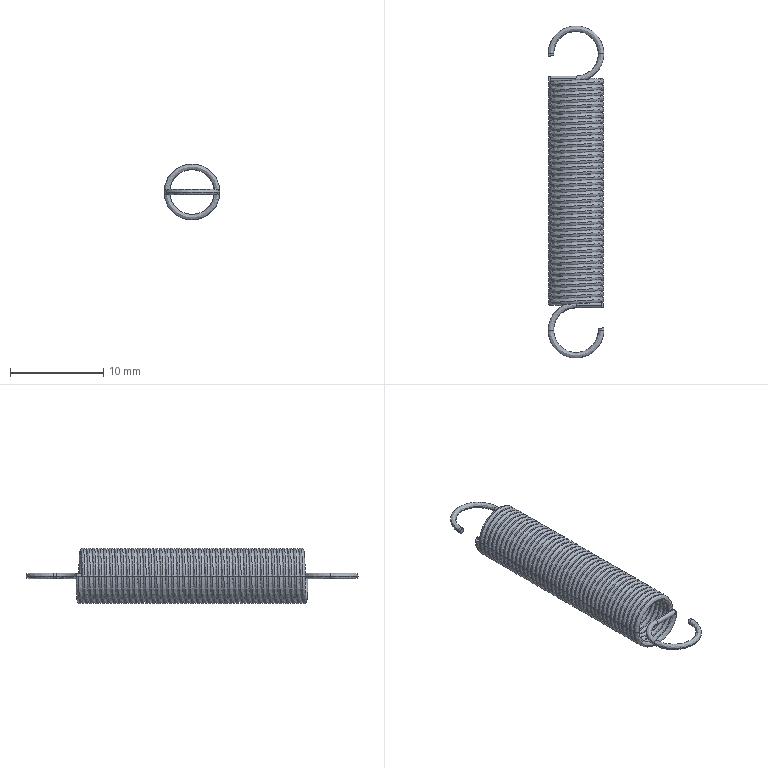Part | SolidWorks | features BaseBody 83 | 83 solids | 344 faces | box 6.01 x 35.7 x 6.018 mm | volume 209.96 mm3 | spline 174 | plane 166 | cylinder 4 | commonest cylinder face diameters 0.6 x4